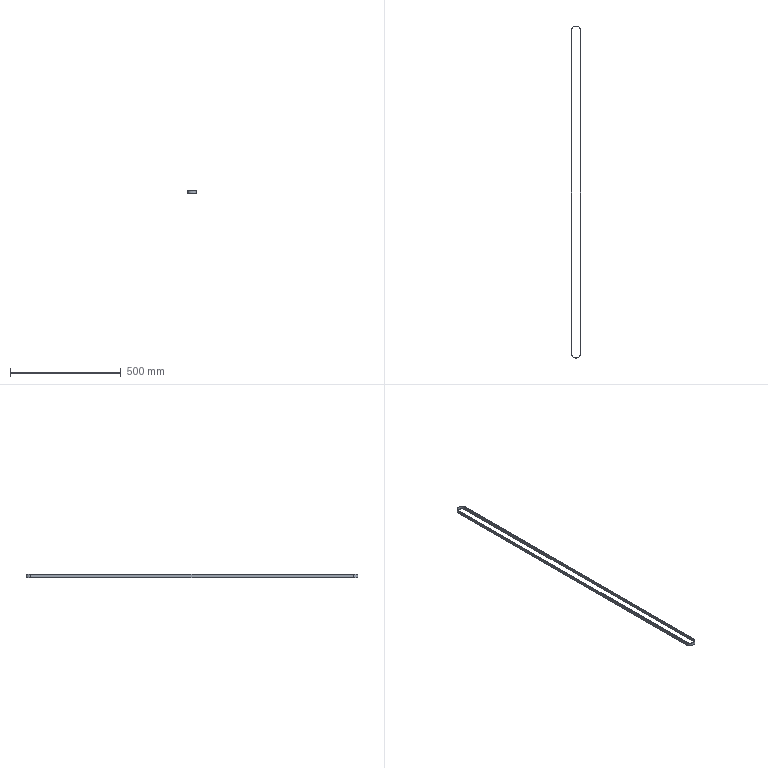Part | 1 solid | 10 faces | box 40.83 x 1496 x 15 mm | volume 45527 mm3 | plane 6 | cylinder 4 | commonest cylinder face diameters 38.83 x2 40.83 x2
STEP:
#1=CARTESIAN_POINT('',(-20.415,0.,7.5));
#2=VERTEX_POINT('',#1);
#3=CARTESIAN_POINT('',(20.415,0.,7.5));
#4=VERTEX_POINT('',#3);
#5=CARTESIAN_POINT('',(0.,0.,7.5));
#6=DIRECTION('',(0.,0.,1.));
#7=DIRECTION('',(-1.,0.,0.));
#8=AXIS2_PLACEMENT_3D('',#5,#6,#7);
#9=CIRCLE('',#8,20.415);
#10=EDGE_CURVE('',#2,#4,#9,.T.);
#11=ORIENTED_EDGE('',*,*,#10,.T.);
#12=CARTESIAN_POINT('',(20.415,1455.,7.5));
#13=VERTEX_POINT('',#12);
#14=CARTESIAN_POINT('',(20.415,0.,7.5));
#15=DIRECTION('',(0.,1.,0.));
#16=VECTOR('',#15,1000.);
#17=LINE('',#14,#16);
#18=EDGE_CURVE('',#4,#13,#17,.T.);
#19=ORIENTED_EDGE('',*,*,#18,.T.);
#20=CARTESIAN_POINT('',(-20.415,1455.,7.5));
#21=VERTEX_POINT('',#20);
#22=CARTESIAN_POINT('',(0.,1455.,7.5));
#23=DIRECTION('',(0.,0.,1.));
#24=DIRECTION('',(-1.,0.,0.));
#25=AXIS2_PLACEMENT_3D('',#22,#23,#24);
#26=CIRCLE('',#25,20.415);
#27=EDGE_CURVE('',#13,#21,#26,.T.);
#28=ORIENTED_EDGE('',*,*,#27,.T.);
#29=CARTESIAN_POINT('',(-20.415,0.,7.5));
#30=DIRECTION('',(0.,-1.,0.));
#31=VECTOR('',#30,1000.);
#32=LINE('',#29,#31);
#33=EDGE_CURVE('',#21,#2,#32,.T.);
#34=ORIENTED_EDGE('',*,*,#33,.T.);
#35=EDGE_LOOP('',(#11,#19,#28,#34));
#36=FACE_OUTER_BOUND('',#35,.T.);
#37=CARTESIAN_POINT('',(-19.415,0.,7.5));
#38=VERTEX_POINT('',#37);
#39=CARTESIAN_POINT('',(19.415,0.,7.5));
#40=VERTEX_POINT('',#39);
#41=CARTESIAN_POINT('',(0.,0.,7.5));
#42=DIRECTION('',(0.,0.,1.));
#43=DIRECTION('',(-1.,0.,0.));
#44=AXIS2_PLACEMENT_3D('',#41,#42,#43);
#45=CIRCLE('',#44,19.415);
#46=EDGE_CURVE('',#38,#40,#45,.T.);
#47=ORIENTED_EDGE('',*,*,#46,.F.);
#48=CARTESIAN_POINT('',(-19.415,1455.,7.5));
#49=VERTEX_POINT('',#48);
#50=CARTESIAN_POINT('',(-19.415,0.,7.5));
#51=DIRECTION('',(0.,-1.,0.));
#52=VECTOR('',#51,1000.);
#53=LINE('',#50,#52);
#54=EDGE_CURVE('',#49,#38,#53,.T.);
#55=ORIENTED_EDGE('',*,*,#54,.F.);
#56=CARTESIAN_POINT('',(19.415,1455.,7.5));
#57=VERTEX_POINT('',#56);
#58=CARTESIAN_POINT('',(0.,1455.,7.5));
#59=DIRECTION('',(0.,0.,1.));
#60=DIRECTION('',(-1.,0.,0.));
#61=AXIS2_PLACEMENT_3D('',#58,#59,#60);
#62=CIRCLE('',#61,19.415);
#63=EDGE_CURVE('',#57,#49,#62,.T.);
#64=ORIENTED_EDGE('',*,*,#63,.F.);
#65=CARTESIAN_POINT('',(19.415,1455.,7.5));
#66=DIRECTION('',(0.,1.,0.));
#67=VECTOR('',#66,1000.);
#68=LINE('',#65,#67);
#69=EDGE_CURVE('',#40,#57,#68,.T.);
#70=ORIENTED_EDGE('',*,*,#69,.F.);
#71=EDGE_LOOP('',(#47,#55,#64,#70));
#72=FACE_BOUND('',#71,.T.);
#73=CARTESIAN_POINT('',(0.,0.,7.5));
#74=DIRECTION('',(0.,0.,-1.));
#75=DIRECTION('',(-1.,0.,0.));
#76=AXIS2_PLACEMENT_3D('',#73,#74,#75);
#77=PLANE('',#76);
#78=ADVANCED_FACE('',(#36,#72),#77,.F.);
#79=CARTESIAN_POINT('',(-20.415,0.,-7.5));
#80=VERTEX_POINT('',#79);
#81=CARTESIAN_POINT('',(20.415,0.,-7.5));
#82=VERTEX_POINT('',#81);
#83=CARTESIAN_POINT('',(0.,0.,-7.5));
#84=DIRECTION('',(0.,0.,1.));
#85=DIRECTION('',(-1.,0.,0.));
#86=AXIS2_PLACEMENT_3D('',#83,#84,#85);
#87=CIRCLE('',#86,20.415);
#88=EDGE_CURVE('',#80,#82,#87,.T.);
#89=ORIENTED_EDGE('',*,*,#88,.F.);
#90=CARTESIAN_POINT('',(-20.415,1455.,-7.5));
#91=VERTEX_POINT('',#90);
#92=CARTESIAN_POINT('',(-20.415,0.,-7.5));
#93=DIRECTION('',(0.,-1.,0.));
#94=VECTOR('',#93,1000.);
#95=LINE('',#92,#94);
#96=EDGE_CURVE('',#91,#80,#95,.T.);
#97=ORIENTED_EDGE('',*,*,#96,.F.);
#98=CARTESIAN_POINT('',(20.415,1455.,-7.5));
#99=VERTEX_POINT('',#98);
#100=CARTESIAN_POINT('',(0.,1455.,-7.5));
#101=DIRECTION('',(0.,0.,1.));
#102=DIRECTION('',(-1.,0.,0.));
#103=AXIS2_PLACEMENT_3D('',#100,#101,#102);
#104=CIRCLE('',#103,20.415);
#105=EDGE_CURVE('',#99,#91,#104,.T.);
#106=ORIENTED_EDGE('',*,*,#105,.F.);
#107=CARTESIAN_POINT('',(20.415,0.,-7.5));
#108=DIRECTION('',(0.,1.,0.));
#109=VECTOR('',#108,1000.);
#110=LINE('',#107,#109);
#111=EDGE_CURVE('',#82,#99,#110,.T.);
#112=ORIENTED_EDGE('',*,*,#111,.F.);
#113=EDGE_LOOP('',(#89,#97,#106,#112));
#114=FACE_OUTER_BOUND('',#113,.T.);
#115=CARTESIAN_POINT('',(-19.415,1455.,-7.5));
#116=VERTEX_POINT('',#115);
#117=CARTESIAN_POINT('',(-19.415,0.,-7.5));
#118=VERTEX_POINT('',#117);
#119=CARTESIAN_POINT('',(-19.415,0.,-7.5));
#120=DIRECTION('',(0.,-1.,0.));
#121=VECTOR('',#120,1000.);
#122=LINE('',#119,#121);
#123=EDGE_CURVE('',#116,#118,#122,.T.);
#124=ORIENTED_EDGE('',*,*,#123,.T.);
#125=CARTESIAN_POINT('',(19.415,0.,-7.5));
#126=VERTEX_POINT('',#125);
#127=CARTESIAN_POINT('',(0.,0.,-7.5));
#128=DIRECTION('',(0.,0.,1.));
#129=DIRECTION('',(-1.,0.,0.));
#130=AXIS2_PLACEMENT_3D('',#127,#128,#129);
#131=CIRCLE('',#130,19.415);
#132=EDGE_CURVE('',#118,#126,#131,.T.);
#133=ORIENTED_EDGE('',*,*,#132,.T.);
#134=CARTESIAN_POINT('',(19.415,1455.,-7.5));
#135=VERTEX_POINT('',#134);
#136=CARTESIAN_POINT('',(19.415,1455.,-7.5));
#137=DIRECTION('',(0.,1.,0.));
#138=VECTOR('',#137,1000.);
#139=LINE('',#136,#138);
#140=EDGE_CURVE('',#126,#135,#139,.T.);
#141=ORIENTED_EDGE('',*,*,#140,.T.);
#142=CARTESIAN_POINT('',(0.,1455.,-7.5));
#143=DIRECTION('',(0.,0.,1.));
#144=DIRECTION('',(-1.,0.,0.));
#145=AXIS2_PLACEMENT_3D('',#142,#143,#144);
#146=CIRCLE('',#145,19.415);
#147=EDGE_CURVE('',#135,#116,#146,.T.);
#148=ORIENTED_EDGE('',*,*,#147,.T.);
#149=EDGE_LOOP('',(#124,#133,#141,#148));
#150=FACE_BOUND('',#149,.T.);
#151=CARTESIAN_POINT('',(0.,0.,-7.5));
#152=DIRECTION('',(0.,0.,-1.));
#153=DIRECTION('',(-1.,0.,0.));
#154=AXIS2_PLACEMENT_3D('',#151,#152,#153);
#155=PLANE('',#154);
#156=ADVANCED_FACE('',(#114,#150),#155,.T.);
#157=ORIENTED_EDGE('',*,*,#88,.T.);
#158=CARTESIAN_POINT('',(20.415,0.,7.5));
#159=DIRECTION('',(0.,0.,-1.));
#160=VECTOR('',#159,1000.);
#161=LINE('',#158,#160);
#162=EDGE_CURVE('',#4,#82,#161,.T.);
#163=ORIENTED_EDGE('',*,*,#162,.F.);
#164=ORIENTED_EDGE('',*,*,#10,.F.);
#165=CARTESIAN_POINT('',(-20.415,0.,7.5));
#166=DIRECTION('',(0.,0.,-1.));
#167=VECTOR('',#166,1000.);
#168=LINE('',#165,#167);
#169=EDGE_CURVE('',#2,#80,#168,.T.);
#170=ORIENTED_EDGE('',*,*,#169,.T.);
#171=EDGE_LOOP('',(#157,#163,#164,#170));
#172=FACE_OUTER_BOUND('',#171,.T.);
#173=CARTESIAN_POINT('',(0.,0.,7.5));
#174=DIRECTION('',(0.,0.,-1.));
#175=DIRECTION('',(-1.,0.,0.));
#176=AXIS2_PLACEMENT_3D('',#173,#174,#175);
#177=CYLINDRICAL_SURFACE('',#176,20.415);
#178=ADVANCED_FACE('',(#172),#177,.T.);
#179=ORIENTED_EDGE('',*,*,#111,.T.);
#180=CARTESIAN_POINT('',(20.415,1455.,7.5));
#181=DIRECTION('',(0.,0.,-1.));
#182=VECTOR('',#181,1000.);
#183=LINE('',#180,#182);
#184=EDGE_CURVE('',#13,#99,#183,.T.);
#185=ORIENTED_EDGE('',*,*,#184,.F.);
#186=ORIENTED_EDGE('',*,*,#18,.F.);
#187=ORIENTED_EDGE('',*,*,#162,.T.);
#188=EDGE_LOOP('',(#179,#185,#186,#187));
#189=FACE_OUTER_BOUND('',#188,.T.);
#190=CARTESIAN_POINT('',(20.415,0.,7.5));
#191=DIRECTION('',(-1.,0.,0.));
#192=DIRECTION('',(0.,-1.,0.));
#193=AXIS2_PLACEMENT_3D('',#190,#191,#192);
#194=PLANE('',#193);
#195=ADVANCED_FACE('',(#189),#194,.F.);
#196=ORIENTED_EDGE('',*,*,#105,.T.);
#197=CARTESIAN_POINT('',(-20.415,1455.,7.5));
#198=DIRECTION('',(0.,0.,-1.));
#199=VECTOR('',#198,1000.);
#200=LINE('',#197,#199);
#201=EDGE_CURVE('',#21,#91,#200,.T.);
#202=ORIENTED_EDGE('',*,*,#201,.F.);
#203=ORIENTED_EDGE('',*,*,#27,.F.);
#204=ORIENTED_EDGE('',*,*,#184,.T.);
#205=EDGE_LOOP('',(#196,#202,#203,#204));
#206=FACE_OUTER_BOUND('',#205,.T.);
#207=CARTESIAN_POINT('',(0.,1455.,7.5));
#208=DIRECTION('',(0.,0.,-1.));
#209=DIRECTION('',(-1.,0.,0.));
#210=AXIS2_PLACEMENT_3D('',#207,#208,#209);
#211=CYLINDRICAL_SURFACE('',#210,20.415);
#212=ADVANCED_FACE('',(#206),#211,.T.);
#213=ORIENTED_EDGE('',*,*,#96,.T.);
#214=ORIENTED_EDGE('',*,*,#169,.F.);
#215=ORIENTED_EDGE('',*,*,#33,.F.);
#216=ORIENTED_EDGE('',*,*,#201,.T.);
#217=EDGE_LOOP('',(#213,#214,#215,#216));
#218=FACE_OUTER_BOUND('',#217,.T.);
#219=CARTESIAN_POINT('',(-20.415,0.,7.5));
#220=DIRECTION('',(1.,0.,0.));
#221=DIRECTION('',(0.,1.,0.));
#222=AXIS2_PLACEMENT_3D('',#219,#220,#221);
#223=PLANE('',#222);
#224=ADVANCED_FACE('',(#218),#223,.F.);
#225=ORIENTED_EDGE('',*,*,#132,.F.);
#226=CARTESIAN_POINT('',(-19.415,0.,7.5));
#227=DIRECTION('',(0.,0.,-1.));
#228=VECTOR('',#227,1000.);
#229=LINE('',#226,#228);
#230=EDGE_CURVE('',#38,#118,#229,.T.);
#231=ORIENTED_EDGE('',*,*,#230,.F.);
#232=ORIENTED_EDGE('',*,*,#46,.T.);
#233=CARTESIAN_POINT('',(19.415,0.,7.5));
#234=DIRECTION('',(0.,0.,-1.));
#235=VECTOR('',#234,1000.);
#236=LINE('',#233,#235);
#237=EDGE_CURVE('',#40,#126,#236,.T.);
#238=ORIENTED_EDGE('',*,*,#237,.T.);
#239=EDGE_LOOP('',(#225,#231,#232,#238));
#240=FACE_OUTER_BOUND('',#239,.T.);
#241=CARTESIAN_POINT('',(0.,0.,7.5));
#242=DIRECTION('',(0.,0.,-1.));
#243=DIRECTION('',(-1.,0.,0.));
#244=AXIS2_PLACEMENT_3D('',#241,#242,#243);
#245=CYLINDRICAL_SURFACE('',#244,19.415);
#246=ADVANCED_FACE('',(#240),#245,.F.);
#247=ORIENTED_EDGE('',*,*,#140,.F.);
#248=ORIENTED_EDGE('',*,*,#237,.F.);
#249=ORIENTED_EDGE('',*,*,#69,.T.);
#250=CARTESIAN_POINT('',(19.415,1455.,7.5));
#251=DIRECTION('',(0.,0.,-1.));
#252=VECTOR('',#251,1000.);
#253=LINE('',#250,#252);
#254=EDGE_CURVE('',#57,#135,#253,.T.);
#255=ORIENTED_EDGE('',*,*,#254,.T.);
#256=EDGE_LOOP('',(#247,#248,#249,#255));
#257=FACE_OUTER_BOUND('',#256,.T.);
#258=CARTESIAN_POINT('',(19.415,1455.,7.5));
#259=DIRECTION('',(-1.,0.,0.));
#260=DIRECTION('',(0.,-1.,0.));
#261=AXIS2_PLACEMENT_3D('',#258,#259,#260);
#262=PLANE('',#261);
#263=ADVANCED_FACE('',(#257),#262,.T.);
#264=ORIENTED_EDGE('',*,*,#147,.F.);
#265=ORIENTED_EDGE('',*,*,#254,.F.);
#266=ORIENTED_EDGE('',*,*,#63,.T.);
#267=CARTESIAN_POINT('',(-19.415,1455.,7.5));
#268=DIRECTION('',(0.,0.,-1.));
#269=VECTOR('',#268,1000.);
#270=LINE('',#267,#269);
#271=EDGE_CURVE('',#49,#116,#270,.T.);
#272=ORIENTED_EDGE('',*,*,#271,.T.);
#273=EDGE_LOOP('',(#264,#265,#266,#272));
#274=FACE_OUTER_BOUND('',#273,.T.);
#275=CARTESIAN_POINT('',(0.,1455.,7.5));
#276=DIRECTION('',(0.,0.,-1.));
#277=DIRECTION('',(-1.,0.,0.));
#278=AXIS2_PLACEMENT_3D('',#275,#276,#277);
#279=CYLINDRICAL_SURFACE('',#278,19.415);
#280=ADVANCED_FACE('',(#274),#279,.F.);
#281=ORIENTED_EDGE('',*,*,#123,.F.);
#282=ORIENTED_EDGE('',*,*,#271,.F.);
#283=ORIENTED_EDGE('',*,*,#54,.T.);
#284=ORIENTED_EDGE('',*,*,#230,.T.);
#285=EDGE_LOOP('',(#281,#282,#283,#284));
#286=FACE_OUTER_BOUND('',#285,.T.);
#287=CARTESIAN_POINT('',(-19.415,0.,7.5));
#288=DIRECTION('',(1.,0.,0.));
#289=DIRECTION('',(0.,1.,0.));
#290=AXIS2_PLACEMENT_3D('',#287,#288,#289);
#291=PLANE('',#290);
#292=ADVANCED_FACE('',(#286),#291,.T.);
#293=CLOSED_SHELL('',(#78,#156,#178,#195,#212,#224,#246,#263,#280,#292));
#294=MANIFOLD_SOLID_BREP('',#293);
#295=CARTESIAN_POINT('',(0.,0.,0.));
#296=DIRECTION('',(0.,0.,1.));
#297=DIRECTION('',(1.,0.,0.));
#298=AXIS2_PLACEMENT_3D('',#295,#296,#297);
#299=(LENGTH_UNIT()NAMED_UNIT(*)SI_UNIT(.MILLI.,.METRE.));
#300=UNCERTAINTY_MEASURE_WITH_UNIT(LENGTH_MEASURE(0.00001),#299,'','');
#301=(NAMED_UNIT(*)PLANE_ANGLE_UNIT()SI_UNIT($,.RADIAN.));
#302=(NAMED_UNIT(*)SI_UNIT($,.STERADIAN.)SOLID_ANGLE_UNIT());
#303=(GEOMETRIC_REPRESENTATION_CONTEXT(3)GLOBAL_UNCERTAINTY_ASSIGNED_CONTEXT((#300))GLOBAL_UNIT_ASSIGNED_CONTEXT((#299,#301,#302))REPRESENTATION_CONTEXT('',''));
#304=ADVANCED_BREP_SHAPE_REPRESENTATION('',(#294,#298),#303);